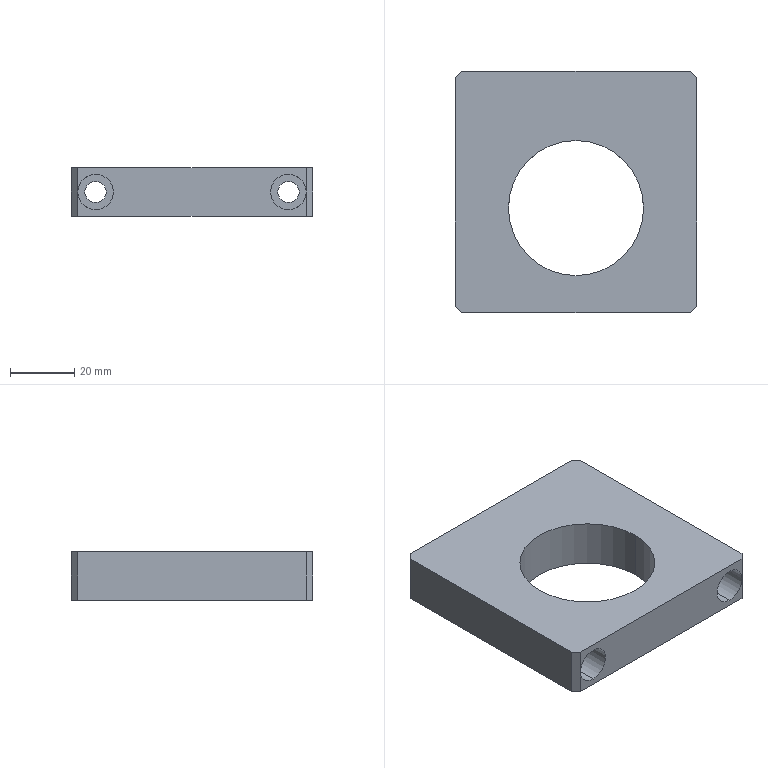Part | STEP file | 1 solid | 22 faces | box 75 x 75 x 15 mm | volume 51651 mm3 | plane 12 | cylinder 10 | commonest cylinder face diameters 6.6 x4 11 x4 42 x2